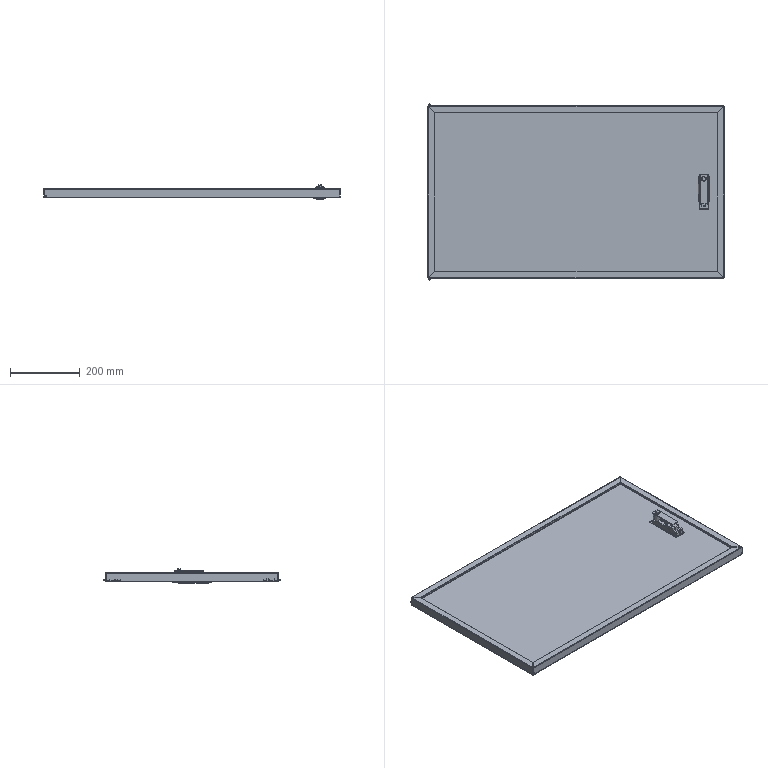Part | SolidWorks | 6 solids | 422 faces | box 851 x 509 x 42.5 mm | volume 870098 mm3 | plane 238 | cylinder 144 | spline 28 | cone 12 | commonest cylinder face diameters 4 x34 1 x17 2 x15 12 x8 8 x6 3 x5